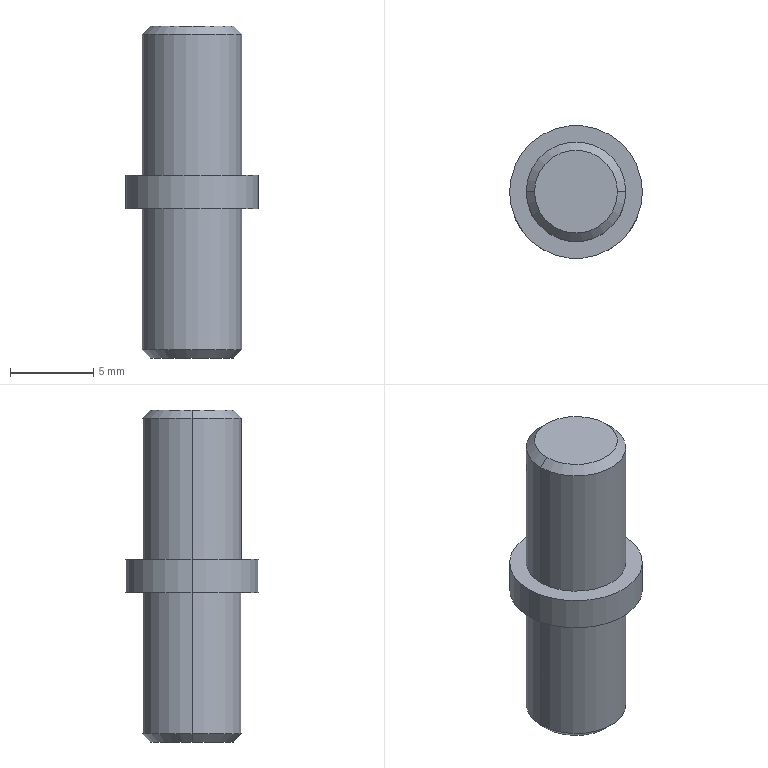Part | SolidWorks | features Chamfer 1, Extrusion 1, ICE 1, MirrorPattern 1 | 1 solid | 14 faces | box 8 x 8 x 20 mm | volume 605.018 mm3 | cylinder 6 | cone 4 | plane 4 | commonest cylinder face diameters 6 x4 8 x2
STEP:
#1=CARTESIAN_POINT('',(2.5,0.,10.));
#2=VERTEX_POINT('',#1);
#3=CARTESIAN_POINT('',(-2.5,0.,10.));
#4=VERTEX_POINT('',#3);
#5=CARTESIAN_POINT('',(0.,0.,10.));
#6=DIRECTION('',(0.,0.,1.));
#7=DIRECTION('',(1.,0.,0.));
#8=AXIS2_PLACEMENT_3D('',#5,#6,#7);
#9=CIRCLE('',#8,2.5);
#10=EDGE_CURVE('',#2,#4,#9,.T.);
#11=ORIENTED_EDGE('',*,*,#10,.F.);
#12=CARTESIAN_POINT('',(3.,0.,9.5));
#13=VERTEX_POINT('',#12);
#14=CARTESIAN_POINT('',(2.5,0.,10.));
#15=DIRECTION('',(0.7071,0.,-0.7071));
#16=VECTOR('',#15,1000.);
#17=LINE('',#14,#16);
#18=EDGE_CURVE('',#2,#13,#17,.T.);
#19=ORIENTED_EDGE('',*,*,#18,.T.);
#20=CARTESIAN_POINT('',(-3.,0.,9.5));
#21=VERTEX_POINT('',#20);
#22=CARTESIAN_POINT('',(0.,0.,9.5));
#23=DIRECTION('',(0.,0.,-1.));
#24=DIRECTION('',(1.,0.,0.));
#25=AXIS2_PLACEMENT_3D('',#22,#23,#24);
#26=CIRCLE('',#25,3.);
#27=EDGE_CURVE('',#21,#13,#26,.T.);
#28=ORIENTED_EDGE('',*,*,#27,.F.);
#29=CARTESIAN_POINT('',(-2.5,0.,10.));
#30=DIRECTION('',(-0.7071,0.,-0.7071));
#31=VECTOR('',#30,1000.);
#32=LINE('',#29,#31);
#33=EDGE_CURVE('',#4,#21,#32,.T.);
#34=ORIENTED_EDGE('',*,*,#33,.F.);
#35=EDGE_LOOP('',(#11,#19,#28,#34));
#36=FACE_OUTER_BOUND('',#35,.T.);
#37=CARTESIAN_POINT('',(0.,0.,10.));
#38=DIRECTION('',(0.,0.,-1.));
#39=DIRECTION('',(-1.,0.,0.));
#40=AXIS2_PLACEMENT_3D('',#37,#38,#39);
#41=CONICAL_SURFACE('',#40,2.5,0.7854);
#42=ADVANCED_FACE('',(#36),#41,.T.);
#43=CARTESIAN_POINT('',(-2.5,0.,-10.));
#44=VERTEX_POINT('',#43);
#45=CARTESIAN_POINT('',(2.5,0.,-10.));
#46=VERTEX_POINT('',#45);
#47=CARTESIAN_POINT('',(0.,0.,-10.));
#48=DIRECTION('',(0.,0.,-1.));
#49=DIRECTION('',(-1.,0.,0.));
#50=AXIS2_PLACEMENT_3D('',#47,#48,#49);
#51=CIRCLE('',#50,2.5);
#52=EDGE_CURVE('',#44,#46,#51,.T.);
#53=ORIENTED_EDGE('',*,*,#52,.F.);
#54=CARTESIAN_POINT('',(-3.,0.,-9.5));
#55=VERTEX_POINT('',#54);
#56=CARTESIAN_POINT('',(-3.,0.,-9.5));
#57=DIRECTION('',(-0.7071,0.,0.7071));
#58=VECTOR('',#57,1000.);
#59=LINE('',#56,#58);
#60=EDGE_CURVE('',#44,#55,#59,.T.);
#61=ORIENTED_EDGE('',*,*,#60,.T.);
#62=CARTESIAN_POINT('',(3.,0.,-9.5));
#63=VERTEX_POINT('',#62);
#64=CARTESIAN_POINT('',(0.,0.,-9.5));
#65=DIRECTION('',(0.,0.,1.));
#66=DIRECTION('',(-1.,0.,0.));
#67=AXIS2_PLACEMENT_3D('',#64,#65,#66);
#68=CIRCLE('',#67,3.);
#69=EDGE_CURVE('',#63,#55,#68,.T.);
#70=ORIENTED_EDGE('',*,*,#69,.F.);
#71=CARTESIAN_POINT('',(3.,0.,-9.5));
#72=DIRECTION('',(0.7071,0.,0.7071));
#73=VECTOR('',#72,1000.);
#74=LINE('',#71,#73);
#75=EDGE_CURVE('',#46,#63,#74,.T.);
#76=ORIENTED_EDGE('',*,*,#75,.F.);
#77=EDGE_LOOP('',(#53,#61,#70,#76));
#78=FACE_OUTER_BOUND('',#77,.T.);
#79=CARTESIAN_POINT('',(0.,0.,-9.5));
#80=DIRECTION('',(0.,0.,1.));
#81=DIRECTION('',(1.,0.,0.));
#82=AXIS2_PLACEMENT_3D('',#79,#80,#81);
#83=CONICAL_SURFACE('',#82,3.,0.7854);
#84=ADVANCED_FACE('',(#78),#83,.T.);
#85=ORIENTED_EDGE('',*,*,#69,.T.);
#86=CARTESIAN_POINT('',(-3.,0.,-1.));
#87=VERTEX_POINT('',#86);
#88=CARTESIAN_POINT('',(-3.,0.,-10.));
#89=DIRECTION('',(0.,0.,1.));
#90=VECTOR('',#89,1000.);
#91=LINE('',#88,#90);
#92=EDGE_CURVE('',#55,#87,#91,.T.);
#93=ORIENTED_EDGE('',*,*,#92,.T.);
#94=CARTESIAN_POINT('',(3.,0.,-1.));
#95=VERTEX_POINT('',#94);
#96=CARTESIAN_POINT('',(0.,0.,-1.));
#97=DIRECTION('',(0.,0.,1.));
#98=DIRECTION('',(1.,0.,0.));
#99=AXIS2_PLACEMENT_3D('',#96,#97,#98);
#100=CIRCLE('',#99,3.);
#101=EDGE_CURVE('',#95,#87,#100,.T.);
#102=ORIENTED_EDGE('',*,*,#101,.F.);
#103=CARTESIAN_POINT('',(3.,0.,-10.));
#104=DIRECTION('',(0.,0.,1.));
#105=VECTOR('',#104,1000.);
#106=LINE('',#103,#105);
#107=EDGE_CURVE('',#63,#95,#106,.T.);
#108=ORIENTED_EDGE('',*,*,#107,.F.);
#109=EDGE_LOOP('',(#85,#93,#102,#108));
#110=FACE_OUTER_BOUND('',#109,.T.);
#111=CARTESIAN_POINT('',(0.,0.,-10.));
#112=DIRECTION('',(0.,0.,1.));
#113=DIRECTION('',(1.,0.,0.));
#114=AXIS2_PLACEMENT_3D('',#111,#112,#113);
#115=CYLINDRICAL_SURFACE('',#114,3.);
#116=ADVANCED_FACE('',(#110),#115,.T.);
#117=ORIENTED_EDGE('',*,*,#27,.T.);
#118=CARTESIAN_POINT('',(3.,0.,1.));
#119=VERTEX_POINT('',#118);
#120=CARTESIAN_POINT('',(3.,0.,10.));
#121=DIRECTION('',(0.,0.,-1.));
#122=VECTOR('',#121,1000.);
#123=LINE('',#120,#122);
#124=EDGE_CURVE('',#13,#119,#123,.T.);
#125=ORIENTED_EDGE('',*,*,#124,.T.);
#126=CARTESIAN_POINT('',(-3.,0.,1.));
#127=VERTEX_POINT('',#126);
#128=CARTESIAN_POINT('',(0.,0.,1.));
#129=DIRECTION('',(0.,0.,1.));
#130=DIRECTION('',(1.,0.,0.));
#131=AXIS2_PLACEMENT_3D('',#128,#129,#130);
#132=CIRCLE('',#131,3.);
#133=EDGE_CURVE('',#119,#127,#132,.T.);
#134=ORIENTED_EDGE('',*,*,#133,.T.);
#135=CARTESIAN_POINT('',(-3.,0.,10.));
#136=DIRECTION('',(0.,0.,-1.));
#137=VECTOR('',#136,1000.);
#138=LINE('',#135,#137);
#139=EDGE_CURVE('',#21,#127,#138,.T.);
#140=ORIENTED_EDGE('',*,*,#139,.F.);
#141=EDGE_LOOP('',(#117,#125,#134,#140));
#142=FACE_OUTER_BOUND('',#141,.T.);
#143=CARTESIAN_POINT('',(0.,0.,10.));
#144=DIRECTION('',(0.,0.,-1.));
#145=DIRECTION('',(-1.,0.,0.));
#146=AXIS2_PLACEMENT_3D('',#143,#144,#145);
#147=CYLINDRICAL_SURFACE('',#146,3.);
#148=ADVANCED_FACE('',(#142),#147,.T.);
#149=CARTESIAN_POINT('',(4.,0.,1.));
#150=VERTEX_POINT('',#149);
#151=CARTESIAN_POINT('',(-4.,0.,1.));
#152=VERTEX_POINT('',#151);
#153=CARTESIAN_POINT('',(0.,0.,1.));
#154=DIRECTION('',(0.,0.,1.));
#155=DIRECTION('',(1.,0.,0.));
#156=AXIS2_PLACEMENT_3D('',#153,#154,#155);
#157=CIRCLE('',#156,4.);
#158=EDGE_CURVE('',#150,#152,#157,.T.);
#159=ORIENTED_EDGE('',*,*,#158,.F.);
#160=CARTESIAN_POINT('',(4.,0.,-1.));
#161=VERTEX_POINT('',#160);
#162=CARTESIAN_POINT('',(4.,0.,1.));
#163=DIRECTION('',(0.,0.,-1.));
#164=VECTOR('',#163,1000.);
#165=LINE('',#162,#164);
#166=EDGE_CURVE('',#150,#161,#165,.T.);
#167=ORIENTED_EDGE('',*,*,#166,.T.);
#168=CARTESIAN_POINT('',(-4.,0.,-1.));
#169=VERTEX_POINT('',#168);
#170=CARTESIAN_POINT('',(0.,0.,-1.));
#171=DIRECTION('',(0.,0.,1.));
#172=DIRECTION('',(1.,0.,0.));
#173=AXIS2_PLACEMENT_3D('',#170,#171,#172);
#174=CIRCLE('',#173,4.);
#175=EDGE_CURVE('',#161,#169,#174,.T.);
#176=ORIENTED_EDGE('',*,*,#175,.T.);
#177=CARTESIAN_POINT('',(-4.,0.,1.));
#178=DIRECTION('',(0.,0.,-1.));
#179=VECTOR('',#178,1000.);
#180=LINE('',#177,#179);
#181=EDGE_CURVE('',#152,#169,#180,.T.);
#182=ORIENTED_EDGE('',*,*,#181,.F.);
#183=EDGE_LOOP('',(#159,#167,#176,#182));
#184=FACE_OUTER_BOUND('',#183,.T.);
#185=CARTESIAN_POINT('',(0.,0.,1.));
#186=DIRECTION('',(0.,0.,-1.));
#187=DIRECTION('',(-1.,0.,0.));
#188=AXIS2_PLACEMENT_3D('',#185,#186,#187);
#189=CYLINDRICAL_SURFACE('',#188,4.);
#190=ADVANCED_FACE('',(#184),#189,.T.);
#191=CARTESIAN_POINT('',(0.,0.,1.));
#192=DIRECTION('',(0.,0.,1.));
#193=DIRECTION('',(1.,0.,0.));
#194=AXIS2_PLACEMENT_3D('',#191,#192,#193);
#195=CIRCLE('',#194,4.);
#196=EDGE_CURVE('',#152,#150,#195,.T.);
#197=ORIENTED_EDGE('',*,*,#196,.T.);
#198=ORIENTED_EDGE('',*,*,#158,.T.);
#199=EDGE_LOOP('',(#197,#198));
#200=FACE_OUTER_BOUND('',#199,.T.);
#201=CARTESIAN_POINT('',(0.,0.,1.));
#202=DIRECTION('',(0.,0.,1.));
#203=DIRECTION('',(1.,0.,0.));
#204=AXIS2_PLACEMENT_3D('',#201,#202,#203);
#205=CIRCLE('',#204,3.);
#206=EDGE_CURVE('',#127,#119,#205,.T.);
#207=ORIENTED_EDGE('',*,*,#206,.F.);
#208=ORIENTED_EDGE('',*,*,#133,.F.);
#209=EDGE_LOOP('',(#207,#208));
#210=FACE_BOUND('',#209,.T.);
#211=CARTESIAN_POINT('',(0.,0.,1.));
#212=DIRECTION('',(0.,0.,1.));
#213=DIRECTION('',(1.,0.,0.));
#214=AXIS2_PLACEMENT_3D('',#211,#212,#213);
#215=PLANE('',#214);
#216=ADVANCED_FACE('',(#200,#210),#215,.T.);
#217=ORIENTED_EDGE('',*,*,#166,.F.);
#218=ORIENTED_EDGE('',*,*,#196,.F.);
#219=ORIENTED_EDGE('',*,*,#181,.T.);
#220=CARTESIAN_POINT('',(0.,0.,-1.));
#221=DIRECTION('',(0.,0.,1.));
#222=DIRECTION('',(1.,0.,0.));
#223=AXIS2_PLACEMENT_3D('',#220,#221,#222);
#224=CIRCLE('',#223,4.);
#225=EDGE_CURVE('',#169,#161,#224,.T.);
#226=ORIENTED_EDGE('',*,*,#225,.T.);
#227=EDGE_LOOP('',(#217,#218,#219,#226));
#228=FACE_OUTER_BOUND('',#227,.T.);
#229=CARTESIAN_POINT('',(0.,0.,1.));
#230=DIRECTION('',(0.,0.,-1.));
#231=DIRECTION('',(-1.,0.,0.));
#232=AXIS2_PLACEMENT_3D('',#229,#230,#231);
#233=CYLINDRICAL_SURFACE('',#232,4.);
#234=ADVANCED_FACE('',(#228),#233,.T.);
#235=ORIENTED_EDGE('',*,*,#101,.T.);
#236=CARTESIAN_POINT('',(0.,0.,-1.));
#237=DIRECTION('',(0.,0.,1.));
#238=DIRECTION('',(1.,0.,0.));
#239=AXIS2_PLACEMENT_3D('',#236,#237,#238);
#240=CIRCLE('',#239,3.);
#241=EDGE_CURVE('',#87,#95,#240,.T.);
#242=ORIENTED_EDGE('',*,*,#241,.T.);
#243=EDGE_LOOP('',(#235,#242));
#244=FACE_BOUND('',#243,.T.);
#245=ORIENTED_EDGE('',*,*,#225,.F.);
#246=ORIENTED_EDGE('',*,*,#175,.F.);
#247=EDGE_LOOP('',(#245,#246));
#248=FACE_OUTER_BOUND('',#247,.T.);
#249=CARTESIAN_POINT('',(0.,0.,-1.));
#250=DIRECTION('',(0.,0.,1.));
#251=DIRECTION('',(1.,0.,0.));
#252=AXIS2_PLACEMENT_3D('',#249,#250,#251);
#253=PLANE('',#252);
#254=ADVANCED_FACE('',(#244,#248),#253,.F.);
#255=ORIENTED_EDGE('',*,*,#124,.F.);
#256=CARTESIAN_POINT('',(0.,0.,9.5));
#257=DIRECTION('',(0.,0.,-1.));
#258=DIRECTION('',(1.,0.,0.));
#259=AXIS2_PLACEMENT_3D('',#256,#257,#258);
#260=CIRCLE('',#259,3.);
#261=EDGE_CURVE('',#13,#21,#260,.T.);
#262=ORIENTED_EDGE('',*,*,#261,.T.);
#263=ORIENTED_EDGE('',*,*,#139,.T.);
#264=ORIENTED_EDGE('',*,*,#206,.T.);
#265=EDGE_LOOP('',(#255,#262,#263,#264));
#266=FACE_OUTER_BOUND('',#265,.T.);
#267=CARTESIAN_POINT('',(0.,0.,10.));
#268=DIRECTION('',(0.,0.,-1.));
#269=DIRECTION('',(-1.,0.,0.));
#270=AXIS2_PLACEMENT_3D('',#267,#268,#269);
#271=CYLINDRICAL_SURFACE('',#270,3.);
#272=ADVANCED_FACE('',(#266),#271,.T.);
#273=CARTESIAN_POINT('',(0.,0.,10.));
#274=DIRECTION('',(0.,0.,1.));
#275=DIRECTION('',(1.,0.,0.));
#276=AXIS2_PLACEMENT_3D('',#273,#274,#275);
#277=CIRCLE('',#276,2.5);
#278=EDGE_CURVE('',#4,#2,#277,.T.);
#279=ORIENTED_EDGE('',*,*,#278,.T.);
#280=ORIENTED_EDGE('',*,*,#10,.T.);
#281=EDGE_LOOP('',(#279,#280));
#282=FACE_OUTER_BOUND('',#281,.T.);
#283=CARTESIAN_POINT('',(0.,0.,10.));
#284=DIRECTION('',(0.,0.,1.));
#285=DIRECTION('',(1.,0.,0.));
#286=AXIS2_PLACEMENT_3D('',#283,#284,#285);
#287=PLANE('',#286);
#288=ADVANCED_FACE('',(#282),#287,.T.);
#289=ORIENTED_EDGE('',*,*,#92,.F.);
#290=CARTESIAN_POINT('',(0.,0.,-9.5));
#291=DIRECTION('',(0.,0.,1.));
#292=DIRECTION('',(-1.,0.,0.));
#293=AXIS2_PLACEMENT_3D('',#290,#291,#292);
#294=CIRCLE('',#293,3.);
#295=EDGE_CURVE('',#55,#63,#294,.T.);
#296=ORIENTED_EDGE('',*,*,#295,.T.);
#297=ORIENTED_EDGE('',*,*,#107,.T.);
#298=ORIENTED_EDGE('',*,*,#241,.F.);
#299=EDGE_LOOP('',(#289,#296,#297,#298));
#300=FACE_OUTER_BOUND('',#299,.T.);
#301=CARTESIAN_POINT('',(0.,0.,-10.));
#302=DIRECTION('',(0.,0.,1.));
#303=DIRECTION('',(1.,0.,0.));
#304=AXIS2_PLACEMENT_3D('',#301,#302,#303);
#305=CYLINDRICAL_SURFACE('',#304,3.);
#306=ADVANCED_FACE('',(#300),#305,.T.);
#307=CARTESIAN_POINT('',(0.,0.,-10.));
#308=DIRECTION('',(0.,0.,-1.));
#309=DIRECTION('',(-1.,0.,0.));
#310=AXIS2_PLACEMENT_3D('',#307,#308,#309);
#311=CIRCLE('',#310,2.5);
#312=EDGE_CURVE('',#46,#44,#311,.T.);
#313=ORIENTED_EDGE('',*,*,#312,.T.);
#314=ORIENTED_EDGE('',*,*,#52,.T.);
#315=EDGE_LOOP('',(#313,#314));
#316=FACE_OUTER_BOUND('',#315,.T.);
#317=CARTESIAN_POINT('',(0.,0.,-10.));
#318=DIRECTION('',(0.,0.,-1.));
#319=DIRECTION('',(1.,0.,0.));
#320=AXIS2_PLACEMENT_3D('',#317,#318,#319);
#321=PLANE('',#320);
#322=ADVANCED_FACE('',(#316),#321,.T.);
#323=ORIENTED_EDGE('',*,*,#60,.F.);
#324=ORIENTED_EDGE('',*,*,#312,.F.);
#325=ORIENTED_EDGE('',*,*,#75,.T.);
#326=ORIENTED_EDGE('',*,*,#295,.F.);
#327=EDGE_LOOP('',(#323,#324,#325,#326));
#328=FACE_OUTER_BOUND('',#327,.T.);
#329=CARTESIAN_POINT('',(0.,0.,-9.5));
#330=DIRECTION('',(0.,0.,1.));
#331=DIRECTION('',(1.,0.,0.));
#332=AXIS2_PLACEMENT_3D('',#329,#330,#331);
#333=CONICAL_SURFACE('',#332,3.,0.7854);
#334=ADVANCED_FACE('',(#328),#333,.T.);
#335=ORIENTED_EDGE('',*,*,#18,.F.);
#336=ORIENTED_EDGE('',*,*,#278,.F.);
#337=ORIENTED_EDGE('',*,*,#33,.T.);
#338=ORIENTED_EDGE('',*,*,#261,.F.);
#339=EDGE_LOOP('',(#335,#336,#337,#338));
#340=FACE_OUTER_BOUND('',#339,.T.);
#341=CARTESIAN_POINT('',(0.,0.,10.));
#342=DIRECTION('',(0.,0.,-1.));
#343=DIRECTION('',(-1.,0.,0.));
#344=AXIS2_PLACEMENT_3D('',#341,#342,#343);
#345=CONICAL_SURFACE('',#344,2.5,0.7854);
#346=ADVANCED_FACE('',(#340),#345,.T.);
#347=CLOSED_SHELL('',(#42,#84,#116,#148,#190,#216,#234,#254,#272,#288,#306,#322,#334,#346));
#348=MANIFOLD_SOLID_BREP('',#347);
#349=CARTESIAN_POINT('',(0.,0.,0.));
#350=DIRECTION('',(0.,0.,1.));
#351=DIRECTION('',(1.,0.,0.));
#352=AXIS2_PLACEMENT_3D('',#349,#350,#351);
#353=(LENGTH_UNIT()NAMED_UNIT(*)SI_UNIT(.MILLI.,.METRE.));
#354=UNCERTAINTY_MEASURE_WITH_UNIT(LENGTH_MEASURE(0.00001),#353,'','');
#355=(NAMED_UNIT(*)PLANE_ANGLE_UNIT()SI_UNIT($,.RADIAN.));
#356=(NAMED_UNIT(*)SI_UNIT($,.STERADIAN.)SOLID_ANGLE_UNIT());
#357=(GEOMETRIC_REPRESENTATION_CONTEXT(3)GLOBAL_UNCERTAINTY_ASSIGNED_CONTEXT((#354))GLOBAL_UNIT_ASSIGNED_CONTEXT((#353,#355,#356))REPRESENTATION_CONTEXT('',''));
#358=ADVANCED_BREP_SHAPE_REPRESENTATION('',(#348,#352),#357);